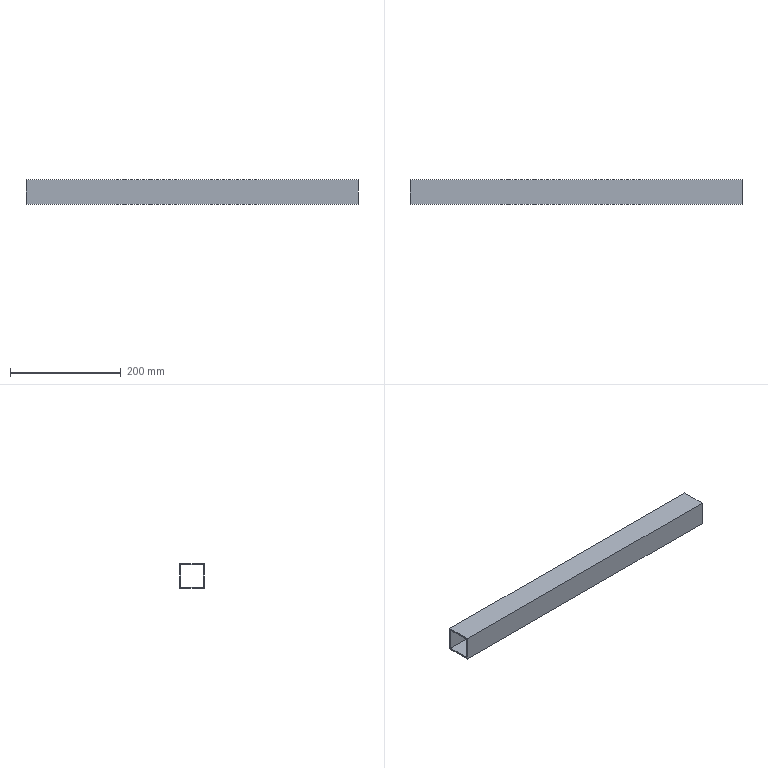Part | STEP file | MB-360X600 | 1 solid | 10 faces | box 600 x 45 x 45 mm | volume 255000 mm3 | plane 10
STEP:
#1=CARTESIAN_POINT('',(0.,42.5,2.5));
#2=VERTEX_POINT('',#1);
#3=CARTESIAN_POINT('',(0.,2.5,2.5));
#4=VERTEX_POINT('',#3);
#5=CARTESIAN_POINT('',(0.,2.5,2.5));
#6=DIRECTION('',(0.,-1.,0.));
#7=VECTOR('',#6,1000.);
#8=LINE('',#5,#7);
#9=EDGE_CURVE('',#2,#4,#8,.T.);
#10=ORIENTED_EDGE('',*,*,#9,.F.);
#11=CARTESIAN_POINT('',(0.,42.5,42.5));
#12=VERTEX_POINT('',#11);
#13=CARTESIAN_POINT('',(0.,42.5,2.5));
#14=DIRECTION('',(0.,0.,-1.));
#15=VECTOR('',#14,1000.);
#16=LINE('',#13,#15);
#17=EDGE_CURVE('',#12,#2,#16,.T.);
#18=ORIENTED_EDGE('',*,*,#17,.F.);
#19=CARTESIAN_POINT('',(0.,2.5,42.5));
#20=VERTEX_POINT('',#19);
#21=CARTESIAN_POINT('',(0.,42.5,42.5));
#22=DIRECTION('',(0.,1.,0.));
#23=VECTOR('',#22,1000.);
#24=LINE('',#21,#23);
#25=EDGE_CURVE('',#20,#12,#24,.T.);
#26=ORIENTED_EDGE('',*,*,#25,.F.);
#27=CARTESIAN_POINT('',(0.,2.5,42.5));
#28=DIRECTION('',(0.,0.,1.));
#29=VECTOR('',#28,1000.);
#30=LINE('',#27,#29);
#31=EDGE_CURVE('',#4,#20,#30,.T.);
#32=ORIENTED_EDGE('',*,*,#31,.F.);
#33=EDGE_LOOP('',(#10,#18,#26,#32));
#34=FACE_BOUND('',#33,.T.);
#35=CARTESIAN_POINT('',(0.,0.,45.));
#36=VERTEX_POINT('',#35);
#37=CARTESIAN_POINT('',(0.,0.,0.));
#38=VERTEX_POINT('',#37);
#39=CARTESIAN_POINT('',(0.,0.,45.));
#40=DIRECTION('',(0.,0.,-1.));
#41=VECTOR('',#40,1000.);
#42=LINE('',#39,#41);
#43=EDGE_CURVE('',#36,#38,#42,.T.);
#44=ORIENTED_EDGE('',*,*,#43,.F.);
#45=CARTESIAN_POINT('',(0.,45.,45.));
#46=VERTEX_POINT('',#45);
#47=CARTESIAN_POINT('',(0.,45.,45.));
#48=DIRECTION('',(0.,-1.,0.));
#49=VECTOR('',#48,1000.);
#50=LINE('',#47,#49);
#51=EDGE_CURVE('',#46,#36,#50,.T.);
#52=ORIENTED_EDGE('',*,*,#51,.F.);
#53=CARTESIAN_POINT('',(0.,45.,0.));
#54=VERTEX_POINT('',#53);
#55=CARTESIAN_POINT('',(0.,45.,0.));
#56=DIRECTION('',(0.,0.,1.));
#57=VECTOR('',#56,1000.);
#58=LINE('',#55,#57);
#59=EDGE_CURVE('',#54,#46,#58,.T.);
#60=ORIENTED_EDGE('',*,*,#59,.F.);
#61=CARTESIAN_POINT('',(0.,0.,0.));
#62=DIRECTION('',(0.,1.,0.));
#63=VECTOR('',#62,1000.);
#64=LINE('',#61,#63);
#65=EDGE_CURVE('',#38,#54,#64,.T.);
#66=ORIENTED_EDGE('',*,*,#65,.F.);
#67=EDGE_LOOP('',(#44,#52,#60,#66));
#68=FACE_OUTER_BOUND('',#67,.T.);
#69=CARTESIAN_POINT('',(0.,22.5,22.5));
#70=DIRECTION('',(1.,0.,0.));
#71=DIRECTION('',(0.,1.,0.));
#72=AXIS2_PLACEMENT_3D('',#69,#70,#71);
#73=PLANE('',#72);
#74=ADVANCED_FACE('',(#34,#68),#73,.F.);
#75=CARTESIAN_POINT('',(600.,42.5,2.5));
#76=VERTEX_POINT('',#75);
#77=CARTESIAN_POINT('',(600.,2.5,2.5));
#78=VERTEX_POINT('',#77);
#79=CARTESIAN_POINT('',(600.,2.5,2.5));
#80=DIRECTION('',(0.,-1.,0.));
#81=VECTOR('',#80,1000.);
#82=LINE('',#79,#81);
#83=EDGE_CURVE('',#76,#78,#82,.T.);
#84=ORIENTED_EDGE('',*,*,#83,.T.);
#85=CARTESIAN_POINT('',(600.,2.5,42.5));
#86=VERTEX_POINT('',#85);
#87=CARTESIAN_POINT('',(600.,2.5,42.5));
#88=DIRECTION('',(0.,0.,1.));
#89=VECTOR('',#88,1000.);
#90=LINE('',#87,#89);
#91=EDGE_CURVE('',#78,#86,#90,.T.);
#92=ORIENTED_EDGE('',*,*,#91,.T.);
#93=CARTESIAN_POINT('',(600.,42.5,42.5));
#94=VERTEX_POINT('',#93);
#95=CARTESIAN_POINT('',(600.,42.5,42.5));
#96=DIRECTION('',(0.,1.,0.));
#97=VECTOR('',#96,1000.);
#98=LINE('',#95,#97);
#99=EDGE_CURVE('',#86,#94,#98,.T.);
#100=ORIENTED_EDGE('',*,*,#99,.T.);
#101=CARTESIAN_POINT('',(600.,42.5,2.5));
#102=DIRECTION('',(0.,0.,-1.));
#103=VECTOR('',#102,1000.);
#104=LINE('',#101,#103);
#105=EDGE_CURVE('',#94,#76,#104,.T.);
#106=ORIENTED_EDGE('',*,*,#105,.T.);
#107=EDGE_LOOP('',(#84,#92,#100,#106));
#108=FACE_BOUND('',#107,.T.);
#109=CARTESIAN_POINT('',(600.,0.,45.));
#110=VERTEX_POINT('',#109);
#111=CARTESIAN_POINT('',(600.,0.,0.));
#112=VERTEX_POINT('',#111);
#113=CARTESIAN_POINT('',(600.,0.,45.));
#114=DIRECTION('',(0.,0.,-1.));
#115=VECTOR('',#114,1000.);
#116=LINE('',#113,#115);
#117=EDGE_CURVE('',#110,#112,#116,.T.);
#118=ORIENTED_EDGE('',*,*,#117,.T.);
#119=CARTESIAN_POINT('',(600.,45.,0.));
#120=VERTEX_POINT('',#119);
#121=CARTESIAN_POINT('',(600.,0.,0.));
#122=DIRECTION('',(0.,1.,0.));
#123=VECTOR('',#122,1000.);
#124=LINE('',#121,#123);
#125=EDGE_CURVE('',#112,#120,#124,.T.);
#126=ORIENTED_EDGE('',*,*,#125,.T.);
#127=CARTESIAN_POINT('',(600.,45.,45.));
#128=VERTEX_POINT('',#127);
#129=CARTESIAN_POINT('',(600.,45.,0.));
#130=DIRECTION('',(0.,0.,1.));
#131=VECTOR('',#130,1000.);
#132=LINE('',#129,#131);
#133=EDGE_CURVE('',#120,#128,#132,.T.);
#134=ORIENTED_EDGE('',*,*,#133,.T.);
#135=CARTESIAN_POINT('',(600.,45.,45.));
#136=DIRECTION('',(0.,-1.,0.));
#137=VECTOR('',#136,1000.);
#138=LINE('',#135,#137);
#139=EDGE_CURVE('',#128,#110,#138,.T.);
#140=ORIENTED_EDGE('',*,*,#139,.T.);
#141=EDGE_LOOP('',(#118,#126,#134,#140));
#142=FACE_OUTER_BOUND('',#141,.T.);
#143=CARTESIAN_POINT('',(600.,22.5,22.5));
#144=DIRECTION('',(1.,0.,0.));
#145=DIRECTION('',(0.,1.,0.));
#146=AXIS2_PLACEMENT_3D('',#143,#144,#145);
#147=PLANE('',#146);
#148=ADVANCED_FACE('',(#108,#142),#147,.T.);
#149=ORIENTED_EDGE('',*,*,#43,.T.);
#150=CARTESIAN_POINT('',(0.,0.,0.));
#151=DIRECTION('',(1.,0.,0.));
#152=VECTOR('',#151,1000.);
#153=LINE('',#150,#152);
#154=EDGE_CURVE('',#38,#112,#153,.T.);
#155=ORIENTED_EDGE('',*,*,#154,.T.);
#156=ORIENTED_EDGE('',*,*,#117,.F.);
#157=CARTESIAN_POINT('',(0.,0.,45.));
#158=DIRECTION('',(1.,0.,0.));
#159=VECTOR('',#158,1000.);
#160=LINE('',#157,#159);
#161=EDGE_CURVE('',#36,#110,#160,.T.);
#162=ORIENTED_EDGE('',*,*,#161,.F.);
#163=EDGE_LOOP('',(#149,#155,#156,#162));
#164=FACE_OUTER_BOUND('',#163,.T.);
#165=CARTESIAN_POINT('',(0.,0.,45.));
#166=DIRECTION('',(0.,-1.,0.));
#167=DIRECTION('',(0.,0.,-1.));
#168=AXIS2_PLACEMENT_3D('',#165,#166,#167);
#169=PLANE('',#168);
#170=ADVANCED_FACE('',(#164),#169,.T.);
#171=ORIENTED_EDGE('',*,*,#65,.T.);
#172=CARTESIAN_POINT('',(0.,45.,0.));
#173=DIRECTION('',(1.,0.,0.));
#174=VECTOR('',#173,1000.);
#175=LINE('',#172,#174);
#176=EDGE_CURVE('',#54,#120,#175,.T.);
#177=ORIENTED_EDGE('',*,*,#176,.T.);
#178=ORIENTED_EDGE('',*,*,#125,.F.);
#179=ORIENTED_EDGE('',*,*,#154,.F.);
#180=EDGE_LOOP('',(#171,#177,#178,#179));
#181=FACE_OUTER_BOUND('',#180,.T.);
#182=CARTESIAN_POINT('',(0.,0.,0.));
#183=DIRECTION('',(0.,0.,-1.));
#184=DIRECTION('',(0.,-1.,0.));
#185=AXIS2_PLACEMENT_3D('',#182,#183,#184);
#186=PLANE('',#185);
#187=ADVANCED_FACE('',(#181),#186,.T.);
#188=ORIENTED_EDGE('',*,*,#59,.T.);
#189=CARTESIAN_POINT('',(0.,45.,45.));
#190=DIRECTION('',(1.,0.,0.));
#191=VECTOR('',#190,1000.);
#192=LINE('',#189,#191);
#193=EDGE_CURVE('',#46,#128,#192,.T.);
#194=ORIENTED_EDGE('',*,*,#193,.T.);
#195=ORIENTED_EDGE('',*,*,#133,.F.);
#196=ORIENTED_EDGE('',*,*,#176,.F.);
#197=EDGE_LOOP('',(#188,#194,#195,#196));
#198=FACE_OUTER_BOUND('',#197,.T.);
#199=CARTESIAN_POINT('',(0.,45.,0.));
#200=DIRECTION('',(0.,1.,0.));
#201=DIRECTION('',(1.,0.,0.));
#202=AXIS2_PLACEMENT_3D('',#199,#200,#201);
#203=PLANE('',#202);
#204=ADVANCED_FACE('',(#198),#203,.T.);
#205=ORIENTED_EDGE('',*,*,#51,.T.);
#206=ORIENTED_EDGE('',*,*,#161,.T.);
#207=ORIENTED_EDGE('',*,*,#139,.F.);
#208=ORIENTED_EDGE('',*,*,#193,.F.);
#209=EDGE_LOOP('',(#205,#206,#207,#208));
#210=FACE_OUTER_BOUND('',#209,.T.);
#211=CARTESIAN_POINT('',(0.,45.,45.));
#212=DIRECTION('',(0.,0.,1.));
#213=DIRECTION('',(1.,0.,0.));
#214=AXIS2_PLACEMENT_3D('',#211,#212,#213);
#215=PLANE('',#214);
#216=ADVANCED_FACE('',(#210),#215,.T.);
#217=ORIENTED_EDGE('',*,*,#9,.T.);
#218=CARTESIAN_POINT('',(0.,2.5,2.5));
#219=DIRECTION('',(1.,0.,0.));
#220=VECTOR('',#219,1000.);
#221=LINE('',#218,#220);
#222=EDGE_CURVE('',#4,#78,#221,.T.);
#223=ORIENTED_EDGE('',*,*,#222,.T.);
#224=ORIENTED_EDGE('',*,*,#83,.F.);
#225=CARTESIAN_POINT('',(0.,42.5,2.5));
#226=DIRECTION('',(1.,0.,0.));
#227=VECTOR('',#226,1000.);
#228=LINE('',#225,#227);
#229=EDGE_CURVE('',#2,#76,#228,.T.);
#230=ORIENTED_EDGE('',*,*,#229,.F.);
#231=EDGE_LOOP('',(#217,#223,#224,#230));
#232=FACE_OUTER_BOUND('',#231,.T.);
#233=CARTESIAN_POINT('',(0.,42.5,2.5));
#234=DIRECTION('',(0.,0.,1.));
#235=DIRECTION('',(1.,0.,0.));
#236=AXIS2_PLACEMENT_3D('',#233,#234,#235);
#237=PLANE('',#236);
#238=ADVANCED_FACE('',(#232),#237,.T.);
#239=ORIENTED_EDGE('',*,*,#31,.T.);
#240=CARTESIAN_POINT('',(0.,2.5,42.5));
#241=DIRECTION('',(1.,0.,0.));
#242=VECTOR('',#241,1000.);
#243=LINE('',#240,#242);
#244=EDGE_CURVE('',#20,#86,#243,.T.);
#245=ORIENTED_EDGE('',*,*,#244,.T.);
#246=ORIENTED_EDGE('',*,*,#91,.F.);
#247=ORIENTED_EDGE('',*,*,#222,.F.);
#248=EDGE_LOOP('',(#239,#245,#246,#247));
#249=FACE_OUTER_BOUND('',#248,.T.);
#250=CARTESIAN_POINT('',(0.,2.5,2.5));
#251=DIRECTION('',(0.,1.,0.));
#252=DIRECTION('',(1.,0.,0.));
#253=AXIS2_PLACEMENT_3D('',#250,#251,#252);
#254=PLANE('',#253);
#255=ADVANCED_FACE('',(#249),#254,.T.);
#256=ORIENTED_EDGE('',*,*,#25,.T.);
#257=CARTESIAN_POINT('',(0.,42.5,42.5));
#258=DIRECTION('',(1.,0.,0.));
#259=VECTOR('',#258,1000.);
#260=LINE('',#257,#259);
#261=EDGE_CURVE('',#12,#94,#260,.T.);
#262=ORIENTED_EDGE('',*,*,#261,.T.);
#263=ORIENTED_EDGE('',*,*,#99,.F.);
#264=ORIENTED_EDGE('',*,*,#244,.F.);
#265=EDGE_LOOP('',(#256,#262,#263,#264));
#266=FACE_OUTER_BOUND('',#265,.T.);
#267=CARTESIAN_POINT('',(0.,2.5,42.5));
#268=DIRECTION('',(0.,0.,-1.));
#269=DIRECTION('',(0.,-1.,0.));
#270=AXIS2_PLACEMENT_3D('',#267,#268,#269);
#271=PLANE('',#270);
#272=ADVANCED_FACE('',(#266),#271,.T.);
#273=ORIENTED_EDGE('',*,*,#17,.T.);
#274=ORIENTED_EDGE('',*,*,#229,.T.);
#275=ORIENTED_EDGE('',*,*,#105,.F.);
#276=ORIENTED_EDGE('',*,*,#261,.F.);
#277=EDGE_LOOP('',(#273,#274,#275,#276));
#278=FACE_OUTER_BOUND('',#277,.T.);
#279=CARTESIAN_POINT('',(0.,42.5,42.5));
#280=DIRECTION('',(0.,-1.,0.));
#281=DIRECTION('',(0.,0.,-1.));
#282=AXIS2_PLACEMENT_3D('',#279,#280,#281);
#283=PLANE('',#282);
#284=ADVANCED_FACE('',(#278),#283,.T.);
#285=CLOSED_SHELL('',(#74,#148,#170,#187,#204,#216,#238,#255,#272,#284));
#286=MANIFOLD_SOLID_BREP('',#285);
#287=CARTESIAN_POINT('',(0.,0.,0.));
#288=DIRECTION('',(0.,0.,1.));
#289=DIRECTION('',(1.,0.,0.));
#290=AXIS2_PLACEMENT_3D('',#287,#288,#289);
#291=(LENGTH_UNIT()NAMED_UNIT(*)SI_UNIT(.MILLI.,.METRE.));
#292=UNCERTAINTY_MEASURE_WITH_UNIT(LENGTH_MEASURE(0.00001),#291,'','');
#293=(NAMED_UNIT(*)PLANE_ANGLE_UNIT()SI_UNIT($,.RADIAN.));
#294=(NAMED_UNIT(*)SI_UNIT($,.STERADIAN.)SOLID_ANGLE_UNIT());
#295=(GEOMETRIC_REPRESENTATION_CONTEXT(3)GLOBAL_UNCERTAINTY_ASSIGNED_CONTEXT((#292))GLOBAL_UNIT_ASSIGNED_CONTEXT((#291,#293,#294))REPRESENTATION_CONTEXT('',''));
#296=ADVANCED_BREP_SHAPE_REPRESENTATION('',(#286,#290),#295);